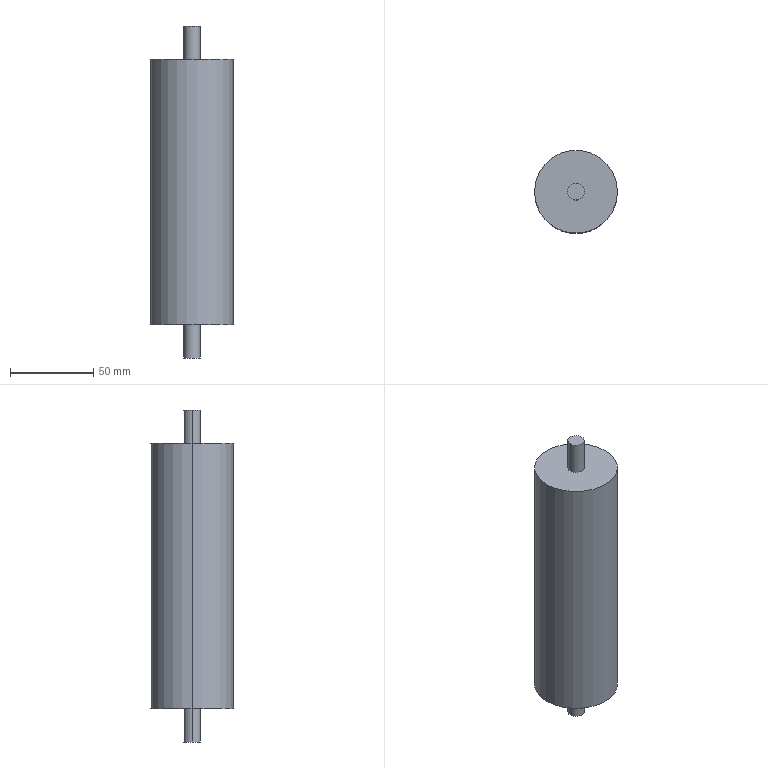Part | SolidWorks | features Extrusion 1, ICE 1, MirrorPattern 1 | 1 solid | 10 faces | box 50 x 50 x 200 mm | volume 317301 mm3 | cylinder 6 | plane 4 | commonest cylinder face diameters 10 x4 50 x2
STEP:
#1=CARTESIAN_POINT('',(-5.,0.,180.));
#2=VERTEX_POINT('',#1);
#3=CARTESIAN_POINT('',(5.,0.,180.));
#4=VERTEX_POINT('',#3);
#5=CARTESIAN_POINT('',(0.,0.,180.));
#6=DIRECTION('',(0.,0.,-1.));
#7=DIRECTION('',(-1.,0.,0.));
#8=AXIS2_PLACEMENT_3D('',#5,#6,#7);
#9=CIRCLE('',#8,5.);
#10=EDGE_CURVE('',#2,#4,#9,.T.);
#11=ORIENTED_EDGE('',*,*,#10,.T.);
#12=CARTESIAN_POINT('',(5.,0.,160.));
#13=VERTEX_POINT('',#12);
#14=CARTESIAN_POINT('',(5.,0.,180.));
#15=DIRECTION('',(0.,0.,-1.));
#16=VECTOR('',#15,1000.);
#17=LINE('',#14,#16);
#18=EDGE_CURVE('',#4,#13,#17,.T.);
#19=ORIENTED_EDGE('',*,*,#18,.T.);
#20=CARTESIAN_POINT('',(-5.,0.,160.));
#21=VERTEX_POINT('',#20);
#22=CARTESIAN_POINT('',(0.,0.,160.));
#23=DIRECTION('',(0.,0.,-1.));
#24=DIRECTION('',(-1.,0.,0.));
#25=AXIS2_PLACEMENT_3D('',#22,#23,#24);
#26=CIRCLE('',#25,5.);
#27=EDGE_CURVE('',#21,#13,#26,.T.);
#28=ORIENTED_EDGE('',*,*,#27,.F.);
#29=CARTESIAN_POINT('',(-5.,0.,180.));
#30=DIRECTION('',(0.,0.,-1.));
#31=VECTOR('',#30,1000.);
#32=LINE('',#29,#31);
#33=EDGE_CURVE('',#2,#21,#32,.T.);
#34=ORIENTED_EDGE('',*,*,#33,.F.);
#35=EDGE_LOOP('',(#11,#19,#28,#34));
#36=FACE_OUTER_BOUND('',#35,.T.);
#37=CARTESIAN_POINT('',(0.,0.,180.));
#38=DIRECTION('',(0.,0.,-1.));
#39=DIRECTION('',(-1.,0.,0.));
#40=AXIS2_PLACEMENT_3D('',#37,#38,#39);
#41=CYLINDRICAL_SURFACE('',#40,5.);
#42=ADVANCED_FACE('',(#36),#41,.T.);
#43=CARTESIAN_POINT('',(-5.,0.,-20.));
#44=VERTEX_POINT('',#43);
#45=CARTESIAN_POINT('',(5.,0.,-20.));
#46=VERTEX_POINT('',#45);
#47=CARTESIAN_POINT('',(0.,0.,-20.));
#48=DIRECTION('',(0.,0.,-1.));
#49=DIRECTION('',(-1.,0.,0.));
#50=AXIS2_PLACEMENT_3D('',#47,#48,#49);
#51=CIRCLE('',#50,5.);
#52=EDGE_CURVE('',#44,#46,#51,.T.);
#53=ORIENTED_EDGE('',*,*,#52,.F.);
#54=CARTESIAN_POINT('',(-5.,0.,0.));
#55=VERTEX_POINT('',#54);
#56=CARTESIAN_POINT('',(-5.,0.,-20.));
#57=DIRECTION('',(0.,0.,1.));
#58=VECTOR('',#57,1000.);
#59=LINE('',#56,#58);
#60=EDGE_CURVE('',#44,#55,#59,.T.);
#61=ORIENTED_EDGE('',*,*,#60,.T.);
#62=CARTESIAN_POINT('',(5.,0.,0.));
#63=VERTEX_POINT('',#62);
#64=CARTESIAN_POINT('',(0.,0.,0.));
#65=DIRECTION('',(0.,0.,-1.));
#66=DIRECTION('',(-1.,0.,0.));
#67=AXIS2_PLACEMENT_3D('',#64,#65,#66);
#68=CIRCLE('',#67,5.);
#69=EDGE_CURVE('',#55,#63,#68,.T.);
#70=ORIENTED_EDGE('',*,*,#69,.T.);
#71=CARTESIAN_POINT('',(5.,0.,-20.));
#72=DIRECTION('',(0.,0.,1.));
#73=VECTOR('',#72,1000.);
#74=LINE('',#71,#73);
#75=EDGE_CURVE('',#46,#63,#74,.T.);
#76=ORIENTED_EDGE('',*,*,#75,.F.);
#77=EDGE_LOOP('',(#53,#61,#70,#76));
#78=FACE_OUTER_BOUND('',#77,.T.);
#79=CARTESIAN_POINT('',(0.,0.,-20.));
#80=DIRECTION('',(0.,0.,1.));
#81=DIRECTION('',(1.,0.,0.));
#82=AXIS2_PLACEMENT_3D('',#79,#80,#81);
#83=CYLINDRICAL_SURFACE('',#82,5.);
#84=ADVANCED_FACE('',(#78),#83,.T.);
#85=CARTESIAN_POINT('',(25.,0.,160.));
#86=VERTEX_POINT('',#85);
#87=CARTESIAN_POINT('',(-25.,0.,160.));
#88=VERTEX_POINT('',#87);
#89=CARTESIAN_POINT('',(0.,0.,160.));
#90=DIRECTION('',(0.,0.,1.));
#91=DIRECTION('',(1.,0.,0.));
#92=AXIS2_PLACEMENT_3D('',#89,#90,#91);
#93=CIRCLE('',#92,25.);
#94=EDGE_CURVE('',#86,#88,#93,.T.);
#95=ORIENTED_EDGE('',*,*,#94,.F.);
#96=CARTESIAN_POINT('',(25.,0.,0.));
#97=VERTEX_POINT('',#96);
#98=CARTESIAN_POINT('',(25.,0.,160.));
#99=DIRECTION('',(0.,0.,-1.));
#100=VECTOR('',#99,1000.);
#101=LINE('',#98,#100);
#102=EDGE_CURVE('',#86,#97,#101,.T.);
#103=ORIENTED_EDGE('',*,*,#102,.T.);
#104=CARTESIAN_POINT('',(-25.,0.,0.));
#105=VERTEX_POINT('',#104);
#106=CARTESIAN_POINT('',(0.,0.,0.));
#107=DIRECTION('',(0.,0.,1.));
#108=DIRECTION('',(1.,0.,0.));
#109=AXIS2_PLACEMENT_3D('',#106,#107,#108);
#110=CIRCLE('',#109,25.);
#111=EDGE_CURVE('',#97,#105,#110,.T.);
#112=ORIENTED_EDGE('',*,*,#111,.T.);
#113=CARTESIAN_POINT('',(-25.,0.,160.));
#114=DIRECTION('',(0.,0.,-1.));
#115=VECTOR('',#114,1000.);
#116=LINE('',#113,#115);
#117=EDGE_CURVE('',#88,#105,#116,.T.);
#118=ORIENTED_EDGE('',*,*,#117,.F.);
#119=EDGE_LOOP('',(#95,#103,#112,#118));
#120=FACE_OUTER_BOUND('',#119,.T.);
#121=CARTESIAN_POINT('',(0.,0.,160.));
#122=DIRECTION('',(0.,0.,-1.));
#123=DIRECTION('',(-1.,0.,0.));
#124=AXIS2_PLACEMENT_3D('',#121,#122,#123);
#125=CYLINDRICAL_SURFACE('',#124,25.);
#126=ADVANCED_FACE('',(#120),#125,.T.);
#127=ORIENTED_EDGE('',*,*,#102,.F.);
#128=CARTESIAN_POINT('',(0.,0.,160.));
#129=DIRECTION('',(0.,0.,1.));
#130=DIRECTION('',(1.,0.,0.));
#131=AXIS2_PLACEMENT_3D('',#128,#129,#130);
#132=CIRCLE('',#131,25.);
#133=EDGE_CURVE('',#88,#86,#132,.T.);
#134=ORIENTED_EDGE('',*,*,#133,.F.);
#135=ORIENTED_EDGE('',*,*,#117,.T.);
#136=CARTESIAN_POINT('',(0.,0.,0.));
#137=DIRECTION('',(0.,0.,1.));
#138=DIRECTION('',(1.,0.,0.));
#139=AXIS2_PLACEMENT_3D('',#136,#137,#138);
#140=CIRCLE('',#139,25.);
#141=EDGE_CURVE('',#105,#97,#140,.T.);
#142=ORIENTED_EDGE('',*,*,#141,.T.);
#143=EDGE_LOOP('',(#127,#134,#135,#142));
#144=FACE_OUTER_BOUND('',#143,.T.);
#145=CARTESIAN_POINT('',(0.,0.,160.));
#146=DIRECTION('',(0.,0.,-1.));
#147=DIRECTION('',(-1.,0.,0.));
#148=AXIS2_PLACEMENT_3D('',#145,#146,#147);
#149=CYLINDRICAL_SURFACE('',#148,25.);
#150=ADVANCED_FACE('',(#144),#149,.T.);
#151=ORIENTED_EDGE('',*,*,#27,.T.);
#152=CARTESIAN_POINT('',(0.,0.,160.));
#153=DIRECTION('',(0.,0.,-1.));
#154=DIRECTION('',(-1.,0.,0.));
#155=AXIS2_PLACEMENT_3D('',#152,#153,#154);
#156=CIRCLE('',#155,5.);
#157=EDGE_CURVE('',#13,#21,#156,.T.);
#158=ORIENTED_EDGE('',*,*,#157,.T.);
#159=EDGE_LOOP('',(#151,#158));
#160=FACE_BOUND('',#159,.T.);
#161=ORIENTED_EDGE('',*,*,#133,.T.);
#162=ORIENTED_EDGE('',*,*,#94,.T.);
#163=EDGE_LOOP('',(#161,#162));
#164=FACE_OUTER_BOUND('',#163,.T.);
#165=CARTESIAN_POINT('',(0.,0.,160.));
#166=DIRECTION('',(0.,0.,1.));
#167=DIRECTION('',(1.,0.,0.));
#168=AXIS2_PLACEMENT_3D('',#165,#166,#167);
#169=PLANE('',#168);
#170=ADVANCED_FACE('',(#160,#164),#169,.T.);
#171=CARTESIAN_POINT('',(0.,0.,0.));
#172=DIRECTION('',(0.,0.,-1.));
#173=DIRECTION('',(-1.,0.,0.));
#174=AXIS2_PLACEMENT_3D('',#171,#172,#173);
#175=CIRCLE('',#174,5.);
#176=EDGE_CURVE('',#63,#55,#175,.T.);
#177=ORIENTED_EDGE('',*,*,#176,.F.);
#178=ORIENTED_EDGE('',*,*,#69,.F.);
#179=EDGE_LOOP('',(#177,#178));
#180=FACE_BOUND('',#179,.T.);
#181=ORIENTED_EDGE('',*,*,#141,.F.);
#182=ORIENTED_EDGE('',*,*,#111,.F.);
#183=EDGE_LOOP('',(#181,#182));
#184=FACE_OUTER_BOUND('',#183,.T.);
#185=CARTESIAN_POINT('',(0.,0.,0.));
#186=DIRECTION('',(0.,0.,1.));
#187=DIRECTION('',(1.,0.,0.));
#188=AXIS2_PLACEMENT_3D('',#185,#186,#187);
#189=PLANE('',#188);
#190=ADVANCED_FACE('',(#180,#184),#189,.F.);
#191=ORIENTED_EDGE('',*,*,#60,.F.);
#192=CARTESIAN_POINT('',(0.,0.,-20.));
#193=DIRECTION('',(0.,0.,-1.));
#194=DIRECTION('',(-1.,0.,0.));
#195=AXIS2_PLACEMENT_3D('',#192,#193,#194);
#196=CIRCLE('',#195,5.);
#197=EDGE_CURVE('',#46,#44,#196,.T.);
#198=ORIENTED_EDGE('',*,*,#197,.F.);
#199=ORIENTED_EDGE('',*,*,#75,.T.);
#200=ORIENTED_EDGE('',*,*,#176,.T.);
#201=EDGE_LOOP('',(#191,#198,#199,#200));
#202=FACE_OUTER_BOUND('',#201,.T.);
#203=CARTESIAN_POINT('',(0.,0.,-20.));
#204=DIRECTION('',(0.,0.,1.));
#205=DIRECTION('',(1.,0.,0.));
#206=AXIS2_PLACEMENT_3D('',#203,#204,#205);
#207=CYLINDRICAL_SURFACE('',#206,5.);
#208=ADVANCED_FACE('',(#202),#207,.T.);
#209=ORIENTED_EDGE('',*,*,#197,.T.);
#210=ORIENTED_EDGE('',*,*,#52,.T.);
#211=EDGE_LOOP('',(#209,#210));
#212=FACE_OUTER_BOUND('',#211,.T.);
#213=CARTESIAN_POINT('',(0.,0.,-20.));
#214=DIRECTION('',(0.,0.,-1.));
#215=DIRECTION('',(-1.,0.,0.));
#216=AXIS2_PLACEMENT_3D('',#213,#214,#215);
#217=PLANE('',#216);
#218=ADVANCED_FACE('',(#212),#217,.T.);
#219=ORIENTED_EDGE('',*,*,#18,.F.);
#220=CARTESIAN_POINT('',(0.,0.,180.));
#221=DIRECTION('',(0.,0.,-1.));
#222=DIRECTION('',(-1.,0.,0.));
#223=AXIS2_PLACEMENT_3D('',#220,#221,#222);
#224=CIRCLE('',#223,5.);
#225=EDGE_CURVE('',#4,#2,#224,.T.);
#226=ORIENTED_EDGE('',*,*,#225,.T.);
#227=ORIENTED_EDGE('',*,*,#33,.T.);
#228=ORIENTED_EDGE('',*,*,#157,.F.);
#229=EDGE_LOOP('',(#219,#226,#227,#228));
#230=FACE_OUTER_BOUND('',#229,.T.);
#231=CARTESIAN_POINT('',(0.,0.,180.));
#232=DIRECTION('',(0.,0.,-1.));
#233=DIRECTION('',(-1.,0.,0.));
#234=AXIS2_PLACEMENT_3D('',#231,#232,#233);
#235=CYLINDRICAL_SURFACE('',#234,5.);
#236=ADVANCED_FACE('',(#230),#235,.T.);
#237=ORIENTED_EDGE('',*,*,#10,.F.);
#238=ORIENTED_EDGE('',*,*,#225,.F.);
#239=EDGE_LOOP('',(#237,#238));
#240=FACE_OUTER_BOUND('',#239,.T.);
#241=CARTESIAN_POINT('',(0.,0.,180.));
#242=DIRECTION('',(0.,0.,1.));
#243=DIRECTION('',(-1.,0.,0.));
#244=AXIS2_PLACEMENT_3D('',#241,#242,#243);
#245=PLANE('',#244);
#246=ADVANCED_FACE('',(#240),#245,.T.);
#247=CLOSED_SHELL('',(#42,#84,#126,#150,#170,#190,#208,#218,#236,#246));
#248=MANIFOLD_SOLID_BREP('',#247);
#249=CARTESIAN_POINT('',(0.,0.,0.));
#250=DIRECTION('',(0.,0.,1.));
#251=DIRECTION('',(1.,0.,0.));
#252=AXIS2_PLACEMENT_3D('',#249,#250,#251);
#253=(LENGTH_UNIT()NAMED_UNIT(*)SI_UNIT(.MILLI.,.METRE.));
#254=UNCERTAINTY_MEASURE_WITH_UNIT(LENGTH_MEASURE(0.00001),#253,'','');
#255=(NAMED_UNIT(*)PLANE_ANGLE_UNIT()SI_UNIT($,.RADIAN.));
#256=(NAMED_UNIT(*)SI_UNIT($,.STERADIAN.)SOLID_ANGLE_UNIT());
#257=(GEOMETRIC_REPRESENTATION_CONTEXT(3)GLOBAL_UNCERTAINTY_ASSIGNED_CONTEXT((#254))GLOBAL_UNIT_ASSIGNED_CONTEXT((#253,#255,#256))REPRESENTATION_CONTEXT('',''));
#258=ADVANCED_BREP_SHAPE_REPRESENTATION('',(#248,#252),#257);